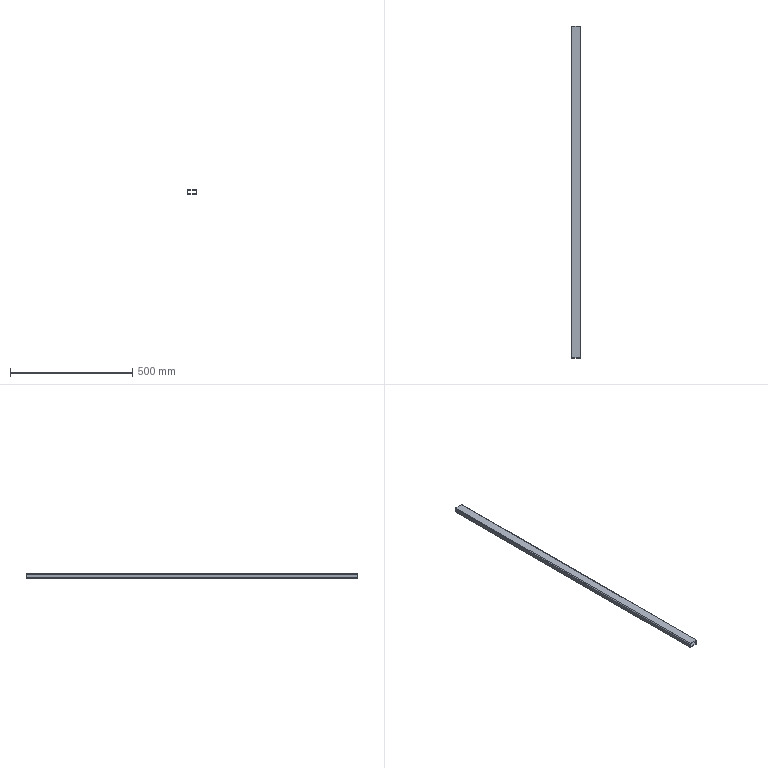Part | SolidWorks | features Extrusion 1 | 1 solid | 18 faces | box 40 x 1360 x 20 mm | volume 334231 mm3 | plane 10 | cylinder 8 | commonest cylinder face diameters 2.3 x4 6.9 x4
STEP:
#1=CARTESIAN_POINT('',(20.,1360.,-6.55));
#2=VERTEX_POINT('',#1);
#3=CARTESIAN_POINT('',(16.55,1360.,-10.));
#4=VERTEX_POINT('',#3);
#5=CARTESIAN_POINT('',(16.55,1360.,-6.55));
#6=DIRECTION('',(0.,1.,0.));
#7=DIRECTION('',(0.,0.,-1.));
#8=AXIS2_PLACEMENT_3D('',#5,#6,#7);
#9=CIRCLE('',#8,3.45);
#10=EDGE_CURVE('',#2,#4,#9,.T.);
#11=ORIENTED_EDGE('',*,*,#10,.T.);
#12=CARTESIAN_POINT('',(-16.55,1360.,-10.));
#13=VERTEX_POINT('',#12);
#14=CARTESIAN_POINT('',(-16.55,1360.,-10.));
#15=DIRECTION('',(-1.,0.,0.));
#16=VECTOR('',#15,1000.);
#17=LINE('',#14,#16);
#18=EDGE_CURVE('',#4,#13,#17,.T.);
#19=ORIENTED_EDGE('',*,*,#18,.T.);
#20=CARTESIAN_POINT('',(-20.,1360.,-6.55));
#21=VERTEX_POINT('',#20);
#22=CARTESIAN_POINT('',(-16.55,1360.,-6.55));
#23=DIRECTION('',(0.,1.,0.));
#24=DIRECTION('',(0.,0.,-1.));
#25=AXIS2_PLACEMENT_3D('',#22,#23,#24);
#26=CIRCLE('',#25,3.45);
#27=EDGE_CURVE('',#13,#21,#26,.T.);
#28=ORIENTED_EDGE('',*,*,#27,.T.);
#29=CARTESIAN_POINT('',(-20.,1360.,6.55));
#30=VERTEX_POINT('',#29);
#31=CARTESIAN_POINT('',(-20.,1360.,6.55));
#32=DIRECTION('',(0.,0.,1.));
#33=VECTOR('',#32,1000.);
#34=LINE('',#31,#33);
#35=EDGE_CURVE('',#21,#30,#34,.T.);
#36=ORIENTED_EDGE('',*,*,#35,.T.);
#37=CARTESIAN_POINT('',(-16.55,1360.,10.));
#38=VERTEX_POINT('',#37);
#39=CARTESIAN_POINT('',(-16.55,1360.,6.55));
#40=DIRECTION('',(0.,1.,0.));
#41=DIRECTION('',(0.,0.,-1.));
#42=AXIS2_PLACEMENT_3D('',#39,#40,#41);
#43=CIRCLE('',#42,3.45);
#44=EDGE_CURVE('',#30,#38,#43,.T.);
#45=ORIENTED_EDGE('',*,*,#44,.T.);
#46=CARTESIAN_POINT('',(16.55,1360.,10.));
#47=VERTEX_POINT('',#46);
#48=CARTESIAN_POINT('',(-16.55,1360.,10.));
#49=DIRECTION('',(1.,0.,0.));
#50=VECTOR('',#49,1000.);
#51=LINE('',#48,#50);
#52=EDGE_CURVE('',#38,#47,#51,.T.);
#53=ORIENTED_EDGE('',*,*,#52,.T.);
#54=CARTESIAN_POINT('',(20.,1360.,6.55));
#55=VERTEX_POINT('',#54);
#56=CARTESIAN_POINT('',(16.55,1360.,6.55));
#57=DIRECTION('',(0.,1.,0.));
#58=DIRECTION('',(0.,0.,1.));
#59=AXIS2_PLACEMENT_3D('',#56,#57,#58);
#60=CIRCLE('',#59,3.45);
#61=EDGE_CURVE('',#47,#55,#60,.T.);
#62=ORIENTED_EDGE('',*,*,#61,.T.);
#63=CARTESIAN_POINT('',(20.,1360.,6.55));
#64=DIRECTION('',(0.,0.,-1.));
#65=VECTOR('',#64,1000.);
#66=LINE('',#63,#65);
#67=EDGE_CURVE('',#55,#2,#66,.T.);
#68=ORIENTED_EDGE('',*,*,#67,.T.);
#69=EDGE_LOOP('',(#11,#19,#28,#36,#45,#53,#62,#68));
#70=FACE_OUTER_BOUND('',#69,.T.);
#71=CARTESIAN_POINT('',(-17.7,1360.,6.55));
#72=VERTEX_POINT('',#71);
#73=CARTESIAN_POINT('',(-16.55,1360.,7.7));
#74=VERTEX_POINT('',#73);
#75=CARTESIAN_POINT('',(-16.55,1360.,6.55));
#76=DIRECTION('',(0.,1.,0.));
#77=DIRECTION('',(0.,0.,-1.));
#78=AXIS2_PLACEMENT_3D('',#75,#76,#77);
#79=CIRCLE('',#78,1.15);
#80=EDGE_CURVE('',#72,#74,#79,.T.);
#81=ORIENTED_EDGE('',*,*,#80,.F.);
#82=CARTESIAN_POINT('',(-17.7,1360.,-6.55));
#83=VERTEX_POINT('',#82);
#84=CARTESIAN_POINT('',(-17.7,1360.,6.55));
#85=DIRECTION('',(0.,0.,1.));
#86=VECTOR('',#85,1000.);
#87=LINE('',#84,#86);
#88=EDGE_CURVE('',#83,#72,#87,.T.);
#89=ORIENTED_EDGE('',*,*,#88,.F.);
#90=CARTESIAN_POINT('',(-16.55,1360.,-7.7));
#91=VERTEX_POINT('',#90);
#92=CARTESIAN_POINT('',(-16.55,1360.,-6.55));
#93=DIRECTION('',(0.,1.,0.));
#94=DIRECTION('',(0.,0.,-1.));
#95=AXIS2_PLACEMENT_3D('',#92,#93,#94);
#96=CIRCLE('',#95,1.15);
#97=EDGE_CURVE('',#91,#83,#96,.T.);
#98=ORIENTED_EDGE('',*,*,#97,.F.);
#99=CARTESIAN_POINT('',(16.55,1360.,-7.7));
#100=VERTEX_POINT('',#99);
#101=CARTESIAN_POINT('',(-16.55,1360.,-7.7));
#102=DIRECTION('',(-1.,0.,0.));
#103=VECTOR('',#102,1000.);
#104=LINE('',#101,#103);
#105=EDGE_CURVE('',#100,#91,#104,.T.);
#106=ORIENTED_EDGE('',*,*,#105,.F.);
#107=CARTESIAN_POINT('',(17.7,1360.,-6.55));
#108=VERTEX_POINT('',#107);
#109=CARTESIAN_POINT('',(16.55,1360.,-6.55));
#110=DIRECTION('',(0.,1.,0.));
#111=DIRECTION('',(0.,0.,-1.));
#112=AXIS2_PLACEMENT_3D('',#109,#110,#111);
#113=CIRCLE('',#112,1.15);
#114=EDGE_CURVE('',#108,#100,#113,.T.);
#115=ORIENTED_EDGE('',*,*,#114,.F.);
#116=CARTESIAN_POINT('',(17.7,1360.,6.55));
#117=VERTEX_POINT('',#116);
#118=CARTESIAN_POINT('',(17.7,1360.,6.55));
#119=DIRECTION('',(0.,0.,-1.));
#120=VECTOR('',#119,1000.);
#121=LINE('',#118,#120);
#122=EDGE_CURVE('',#117,#108,#121,.T.);
#123=ORIENTED_EDGE('',*,*,#122,.F.);
#124=CARTESIAN_POINT('',(16.55,1360.,7.7));
#125=VERTEX_POINT('',#124);
#126=CARTESIAN_POINT('',(16.55,1360.,6.55));
#127=DIRECTION('',(0.,1.,0.));
#128=DIRECTION('',(0.,0.,1.));
#129=AXIS2_PLACEMENT_3D('',#126,#127,#128);
#130=CIRCLE('',#129,1.15);
#131=EDGE_CURVE('',#125,#117,#130,.T.);
#132=ORIENTED_EDGE('',*,*,#131,.F.);
#133=CARTESIAN_POINT('',(-16.55,1360.,7.7));
#134=DIRECTION('',(1.,0.,0.));
#135=VECTOR('',#134,1000.);
#136=LINE('',#133,#135);
#137=EDGE_CURVE('',#74,#125,#136,.T.);
#138=ORIENTED_EDGE('',*,*,#137,.F.);
#139=EDGE_LOOP('',(#81,#89,#98,#106,#115,#123,#132,#138));
#140=FACE_BOUND('',#139,.T.);
#141=CARTESIAN_POINT('',(16.55,1360.,-6.55));
#142=DIRECTION('',(0.,-1.,0.));
#143=DIRECTION('',(0.,0.,-1.));
#144=AXIS2_PLACEMENT_3D('',#141,#142,#143);
#145=PLANE('',#144);
#146=ADVANCED_FACE('',(#70,#140),#145,.F.);
#147=CARTESIAN_POINT('',(20.,0.,-6.55));
#148=VERTEX_POINT('',#147);
#149=CARTESIAN_POINT('',(16.55,0.,-10.));
#150=VERTEX_POINT('',#149);
#151=CARTESIAN_POINT('',(16.55,0.,-6.55));
#152=DIRECTION('',(0.,1.,0.));
#153=DIRECTION('',(0.,0.,-1.));
#154=AXIS2_PLACEMENT_3D('',#151,#152,#153);
#155=CIRCLE('',#154,3.45);
#156=EDGE_CURVE('',#148,#150,#155,.T.);
#157=ORIENTED_EDGE('',*,*,#156,.F.);
#158=CARTESIAN_POINT('',(20.,0.,6.55));
#159=VERTEX_POINT('',#158);
#160=CARTESIAN_POINT('',(20.,0.,6.55));
#161=DIRECTION('',(0.,0.,-1.));
#162=VECTOR('',#161,1000.);
#163=LINE('',#160,#162);
#164=EDGE_CURVE('',#159,#148,#163,.T.);
#165=ORIENTED_EDGE('',*,*,#164,.F.);
#166=CARTESIAN_POINT('',(16.55,0.,10.));
#167=VERTEX_POINT('',#166);
#168=CARTESIAN_POINT('',(16.55,0.,6.55));
#169=DIRECTION('',(0.,1.,0.));
#170=DIRECTION('',(0.,0.,1.));
#171=AXIS2_PLACEMENT_3D('',#168,#169,#170);
#172=CIRCLE('',#171,3.45);
#173=EDGE_CURVE('',#167,#159,#172,.T.);
#174=ORIENTED_EDGE('',*,*,#173,.F.);
#175=CARTESIAN_POINT('',(-16.55,0.,10.));
#176=VERTEX_POINT('',#175);
#177=CARTESIAN_POINT('',(-16.55,0.,10.));
#178=DIRECTION('',(1.,0.,0.));
#179=VECTOR('',#178,1000.);
#180=LINE('',#177,#179);
#181=EDGE_CURVE('',#176,#167,#180,.T.);
#182=ORIENTED_EDGE('',*,*,#181,.F.);
#183=CARTESIAN_POINT('',(-20.,0.,6.55));
#184=VERTEX_POINT('',#183);
#185=CARTESIAN_POINT('',(-16.55,0.,6.55));
#186=DIRECTION('',(0.,1.,0.));
#187=DIRECTION('',(0.,0.,-1.));
#188=AXIS2_PLACEMENT_3D('',#185,#186,#187);
#189=CIRCLE('',#188,3.45);
#190=EDGE_CURVE('',#184,#176,#189,.T.);
#191=ORIENTED_EDGE('',*,*,#190,.F.);
#192=CARTESIAN_POINT('',(-20.,0.,-6.55));
#193=VERTEX_POINT('',#192);
#194=CARTESIAN_POINT('',(-20.,0.,6.55));
#195=DIRECTION('',(0.,0.,1.));
#196=VECTOR('',#195,1000.);
#197=LINE('',#194,#196);
#198=EDGE_CURVE('',#193,#184,#197,.T.);
#199=ORIENTED_EDGE('',*,*,#198,.F.);
#200=CARTESIAN_POINT('',(-16.55,0.,-10.));
#201=VERTEX_POINT('',#200);
#202=CARTESIAN_POINT('',(-16.55,0.,-6.55));
#203=DIRECTION('',(0.,1.,0.));
#204=DIRECTION('',(0.,0.,-1.));
#205=AXIS2_PLACEMENT_3D('',#202,#203,#204);
#206=CIRCLE('',#205,3.45);
#207=EDGE_CURVE('',#201,#193,#206,.T.);
#208=ORIENTED_EDGE('',*,*,#207,.F.);
#209=CARTESIAN_POINT('',(-16.55,0.,-10.));
#210=DIRECTION('',(-1.,0.,0.));
#211=VECTOR('',#210,1000.);
#212=LINE('',#209,#211);
#213=EDGE_CURVE('',#150,#201,#212,.T.);
#214=ORIENTED_EDGE('',*,*,#213,.F.);
#215=EDGE_LOOP('',(#157,#165,#174,#182,#191,#199,#208,#214));
#216=FACE_OUTER_BOUND('',#215,.T.);
#217=CARTESIAN_POINT('',(-17.7,0.,-6.55));
#218=VERTEX_POINT('',#217);
#219=CARTESIAN_POINT('',(-17.7,0.,6.55));
#220=VERTEX_POINT('',#219);
#221=CARTESIAN_POINT('',(-17.7,0.,6.55));
#222=DIRECTION('',(0.,0.,1.));
#223=VECTOR('',#222,1000.);
#224=LINE('',#221,#223);
#225=EDGE_CURVE('',#218,#220,#224,.T.);
#226=ORIENTED_EDGE('',*,*,#225,.T.);
#227=CARTESIAN_POINT('',(-16.55,0.,7.7));
#228=VERTEX_POINT('',#227);
#229=CARTESIAN_POINT('',(-16.55,0.,6.55));
#230=DIRECTION('',(0.,1.,0.));
#231=DIRECTION('',(0.,0.,-1.));
#232=AXIS2_PLACEMENT_3D('',#229,#230,#231);
#233=CIRCLE('',#232,1.15);
#234=EDGE_CURVE('',#220,#228,#233,.T.);
#235=ORIENTED_EDGE('',*,*,#234,.T.);
#236=CARTESIAN_POINT('',(16.55,0.,7.7));
#237=VERTEX_POINT('',#236);
#238=CARTESIAN_POINT('',(-16.55,0.,7.7));
#239=DIRECTION('',(1.,0.,0.));
#240=VECTOR('',#239,1000.);
#241=LINE('',#238,#240);
#242=EDGE_CURVE('',#228,#237,#241,.T.);
#243=ORIENTED_EDGE('',*,*,#242,.T.);
#244=CARTESIAN_POINT('',(17.7,0.,6.55));
#245=VERTEX_POINT('',#244);
#246=CARTESIAN_POINT('',(16.55,0.,6.55));
#247=DIRECTION('',(0.,1.,0.));
#248=DIRECTION('',(0.,0.,1.));
#249=AXIS2_PLACEMENT_3D('',#246,#247,#248);
#250=CIRCLE('',#249,1.15);
#251=EDGE_CURVE('',#237,#245,#250,.T.);
#252=ORIENTED_EDGE('',*,*,#251,.T.);
#253=CARTESIAN_POINT('',(17.7,0.,-6.55));
#254=VERTEX_POINT('',#253);
#255=CARTESIAN_POINT('',(17.7,0.,6.55));
#256=DIRECTION('',(0.,0.,-1.));
#257=VECTOR('',#256,1000.);
#258=LINE('',#255,#257);
#259=EDGE_CURVE('',#245,#254,#258,.T.);
#260=ORIENTED_EDGE('',*,*,#259,.T.);
#261=CARTESIAN_POINT('',(16.55,0.,-7.7));
#262=VERTEX_POINT('',#261);
#263=CARTESIAN_POINT('',(16.55,0.,-6.55));
#264=DIRECTION('',(0.,1.,0.));
#265=DIRECTION('',(0.,0.,-1.));
#266=AXIS2_PLACEMENT_3D('',#263,#264,#265);
#267=CIRCLE('',#266,1.15);
#268=EDGE_CURVE('',#254,#262,#267,.T.);
#269=ORIENTED_EDGE('',*,*,#268,.T.);
#270=CARTESIAN_POINT('',(-16.55,0.,-7.7));
#271=VERTEX_POINT('',#270);
#272=CARTESIAN_POINT('',(-16.55,0.,-7.7));
#273=DIRECTION('',(-1.,0.,0.));
#274=VECTOR('',#273,1000.);
#275=LINE('',#272,#274);
#276=EDGE_CURVE('',#262,#271,#275,.T.);
#277=ORIENTED_EDGE('',*,*,#276,.T.);
#278=CARTESIAN_POINT('',(-16.55,0.,-6.55));
#279=DIRECTION('',(0.,1.,0.));
#280=DIRECTION('',(0.,0.,-1.));
#281=AXIS2_PLACEMENT_3D('',#278,#279,#280);
#282=CIRCLE('',#281,1.15);
#283=EDGE_CURVE('',#271,#218,#282,.T.);
#284=ORIENTED_EDGE('',*,*,#283,.T.);
#285=EDGE_LOOP('',(#226,#235,#243,#252,#260,#269,#277,#284));
#286=FACE_BOUND('',#285,.T.);
#287=CARTESIAN_POINT('',(16.55,0.,-6.55));
#288=DIRECTION('',(0.,-1.,0.));
#289=DIRECTION('',(0.,0.,-1.));
#290=AXIS2_PLACEMENT_3D('',#287,#288,#289);
#291=PLANE('',#290);
#292=ADVANCED_FACE('',(#216,#286),#291,.T.);
#293=ORIENTED_EDGE('',*,*,#156,.T.);
#294=CARTESIAN_POINT('',(16.55,1360.,-10.));
#295=DIRECTION('',(0.,-1.,0.));
#296=VECTOR('',#295,1000.);
#297=LINE('',#294,#296);
#298=EDGE_CURVE('',#4,#150,#297,.T.);
#299=ORIENTED_EDGE('',*,*,#298,.F.);
#300=ORIENTED_EDGE('',*,*,#10,.F.);
#301=CARTESIAN_POINT('',(20.,1360.,-6.55));
#302=DIRECTION('',(0.,-1.,0.));
#303=VECTOR('',#302,1000.);
#304=LINE('',#301,#303);
#305=EDGE_CURVE('',#2,#148,#304,.T.);
#306=ORIENTED_EDGE('',*,*,#305,.T.);
#307=EDGE_LOOP('',(#293,#299,#300,#306));
#308=FACE_OUTER_BOUND('',#307,.T.);
#309=CARTESIAN_POINT('',(16.55,1360.,-6.55));
#310=DIRECTION('',(0.,-1.,0.));
#311=DIRECTION('',(0.,0.,-1.));
#312=AXIS2_PLACEMENT_3D('',#309,#310,#311);
#313=CYLINDRICAL_SURFACE('',#312,3.45);
#314=ADVANCED_FACE('',(#308),#313,.T.);
#315=ORIENTED_EDGE('',*,*,#213,.T.);
#316=CARTESIAN_POINT('',(-16.55,1360.,-10.));
#317=DIRECTION('',(0.,-1.,0.));
#318=VECTOR('',#317,1000.);
#319=LINE('',#316,#318);
#320=EDGE_CURVE('',#13,#201,#319,.T.);
#321=ORIENTED_EDGE('',*,*,#320,.F.);
#322=ORIENTED_EDGE('',*,*,#18,.F.);
#323=ORIENTED_EDGE('',*,*,#298,.T.);
#324=EDGE_LOOP('',(#315,#321,#322,#323));
#325=FACE_OUTER_BOUND('',#324,.T.);
#326=CARTESIAN_POINT('',(-16.55,1360.,-10.));
#327=DIRECTION('',(0.,0.,1.));
#328=DIRECTION('',(1.,0.,0.));
#329=AXIS2_PLACEMENT_3D('',#326,#327,#328);
#330=PLANE('',#329);
#331=ADVANCED_FACE('',(#325),#330,.F.);
#332=ORIENTED_EDGE('',*,*,#207,.T.);
#333=CARTESIAN_POINT('',(-20.,1360.,-6.55));
#334=DIRECTION('',(0.,-1.,0.));
#335=VECTOR('',#334,1000.);
#336=LINE('',#333,#335);
#337=EDGE_CURVE('',#21,#193,#336,.T.);
#338=ORIENTED_EDGE('',*,*,#337,.F.);
#339=ORIENTED_EDGE('',*,*,#27,.F.);
#340=ORIENTED_EDGE('',*,*,#320,.T.);
#341=EDGE_LOOP('',(#332,#338,#339,#340));
#342=FACE_OUTER_BOUND('',#341,.T.);
#343=CARTESIAN_POINT('',(-16.55,1360.,-6.55));
#344=DIRECTION('',(0.,-1.,0.));
#345=DIRECTION('',(0.,0.,-1.));
#346=AXIS2_PLACEMENT_3D('',#343,#344,#345);
#347=CYLINDRICAL_SURFACE('',#346,3.45);
#348=ADVANCED_FACE('',(#342),#347,.T.);
#349=ORIENTED_EDGE('',*,*,#198,.T.);
#350=CARTESIAN_POINT('',(-20.,1360.,6.55));
#351=DIRECTION('',(0.,-1.,0.));
#352=VECTOR('',#351,1000.);
#353=LINE('',#350,#352);
#354=EDGE_CURVE('',#30,#184,#353,.T.);
#355=ORIENTED_EDGE('',*,*,#354,.F.);
#356=ORIENTED_EDGE('',*,*,#35,.F.);
#357=ORIENTED_EDGE('',*,*,#337,.T.);
#358=EDGE_LOOP('',(#349,#355,#356,#357));
#359=FACE_OUTER_BOUND('',#358,.T.);
#360=CARTESIAN_POINT('',(-20.,1360.,6.55));
#361=DIRECTION('',(1.,0.,0.));
#362=DIRECTION('',(0.,0.,-1.));
#363=AXIS2_PLACEMENT_3D('',#360,#361,#362);
#364=PLANE('',#363);
#365=ADVANCED_FACE('',(#359),#364,.F.);
#366=ORIENTED_EDGE('',*,*,#190,.T.);
#367=CARTESIAN_POINT('',(-16.55,1360.,10.));
#368=DIRECTION('',(0.,-1.,0.));
#369=VECTOR('',#368,1000.);
#370=LINE('',#367,#369);
#371=EDGE_CURVE('',#38,#176,#370,.T.);
#372=ORIENTED_EDGE('',*,*,#371,.F.);
#373=ORIENTED_EDGE('',*,*,#44,.F.);
#374=ORIENTED_EDGE('',*,*,#354,.T.);
#375=EDGE_LOOP('',(#366,#372,#373,#374));
#376=FACE_OUTER_BOUND('',#375,.T.);
#377=CARTESIAN_POINT('',(-16.55,1360.,6.55));
#378=DIRECTION('',(0.,-1.,0.));
#379=DIRECTION('',(0.,0.,-1.));
#380=AXIS2_PLACEMENT_3D('',#377,#378,#379);
#381=CYLINDRICAL_SURFACE('',#380,3.45);
#382=ADVANCED_FACE('',(#376),#381,.T.);
#383=ORIENTED_EDGE('',*,*,#181,.T.);
#384=CARTESIAN_POINT('',(16.55,1360.,10.));
#385=DIRECTION('',(0.,-1.,0.));
#386=VECTOR('',#385,1000.);
#387=LINE('',#384,#386);
#388=EDGE_CURVE('',#47,#167,#387,.T.);
#389=ORIENTED_EDGE('',*,*,#388,.F.);
#390=ORIENTED_EDGE('',*,*,#52,.F.);
#391=ORIENTED_EDGE('',*,*,#371,.T.);
#392=EDGE_LOOP('',(#383,#389,#390,#391));
#393=FACE_OUTER_BOUND('',#392,.T.);
#394=CARTESIAN_POINT('',(-16.55,1360.,10.));
#395=DIRECTION('',(0.,0.,-1.));
#396=DIRECTION('',(-1.,0.,0.));
#397=AXIS2_PLACEMENT_3D('',#394,#395,#396);
#398=PLANE('',#397);
#399=ADVANCED_FACE('',(#393),#398,.F.);
#400=ORIENTED_EDGE('',*,*,#173,.T.);
#401=CARTESIAN_POINT('',(20.,1360.,6.55));
#402=DIRECTION('',(0.,-1.,0.));
#403=VECTOR('',#402,1000.);
#404=LINE('',#401,#403);
#405=EDGE_CURVE('',#55,#159,#404,.T.);
#406=ORIENTED_EDGE('',*,*,#405,.F.);
#407=ORIENTED_EDGE('',*,*,#61,.F.);
#408=ORIENTED_EDGE('',*,*,#388,.T.);
#409=EDGE_LOOP('',(#400,#406,#407,#408));
#410=FACE_OUTER_BOUND('',#409,.T.);
#411=CARTESIAN_POINT('',(16.55,1360.,6.55));
#412=DIRECTION('',(0.,-1.,0.));
#413=DIRECTION('',(0.,0.,-1.));
#414=AXIS2_PLACEMENT_3D('',#411,#412,#413);
#415=CYLINDRICAL_SURFACE('',#414,3.45);
#416=ADVANCED_FACE('',(#410),#415,.T.);
#417=ORIENTED_EDGE('',*,*,#164,.T.);
#418=ORIENTED_EDGE('',*,*,#305,.F.);
#419=ORIENTED_EDGE('',*,*,#67,.F.);
#420=ORIENTED_EDGE('',*,*,#405,.T.);
#421=EDGE_LOOP('',(#417,#418,#419,#420));
#422=FACE_OUTER_BOUND('',#421,.T.);
#423=CARTESIAN_POINT('',(20.,1360.,6.55));
#424=DIRECTION('',(-1.,0.,0.));
#425=DIRECTION('',(0.,0.,1.));
#426=AXIS2_PLACEMENT_3D('',#423,#424,#425);
#427=PLANE('',#426);
#428=ADVANCED_FACE('',(#422),#427,.F.);
#429=ORIENTED_EDGE('',*,*,#234,.F.);
#430=CARTESIAN_POINT('',(-17.7,1360.,6.55));
#431=DIRECTION('',(0.,-1.,0.));
#432=VECTOR('',#431,1000.);
#433=LINE('',#430,#432);
#434=EDGE_CURVE('',#72,#220,#433,.T.);
#435=ORIENTED_EDGE('',*,*,#434,.F.);
#436=ORIENTED_EDGE('',*,*,#80,.T.);
#437=CARTESIAN_POINT('',(-16.55,1360.,7.7));
#438=DIRECTION('',(0.,-1.,0.));
#439=VECTOR('',#438,1000.);
#440=LINE('',#437,#439);
#441=EDGE_CURVE('',#74,#228,#440,.T.);
#442=ORIENTED_EDGE('',*,*,#441,.T.);
#443=EDGE_LOOP('',(#429,#435,#436,#442));
#444=FACE_OUTER_BOUND('',#443,.T.);
#445=CARTESIAN_POINT('',(-16.55,1360.,6.55));
#446=DIRECTION('',(0.,-1.,0.));
#447=DIRECTION('',(0.,0.,-1.));
#448=AXIS2_PLACEMENT_3D('',#445,#446,#447);
#449=CYLINDRICAL_SURFACE('',#448,1.15);
#450=ADVANCED_FACE('',(#444),#449,.F.);
#451=ORIENTED_EDGE('',*,*,#242,.F.);
#452=ORIENTED_EDGE('',*,*,#441,.F.);
#453=ORIENTED_EDGE('',*,*,#137,.T.);
#454=CARTESIAN_POINT('',(16.55,1360.,7.7));
#455=DIRECTION('',(0.,-1.,0.));
#456=VECTOR('',#455,1000.);
#457=LINE('',#454,#456);
#458=EDGE_CURVE('',#125,#237,#457,.T.);
#459=ORIENTED_EDGE('',*,*,#458,.T.);
#460=EDGE_LOOP('',(#451,#452,#453,#459));
#461=FACE_OUTER_BOUND('',#460,.T.);
#462=CARTESIAN_POINT('',(-16.55,1360.,7.7));
#463=DIRECTION('',(0.,0.,-1.));
#464=DIRECTION('',(-1.,0.,0.));
#465=AXIS2_PLACEMENT_3D('',#462,#463,#464);
#466=PLANE('',#465);
#467=ADVANCED_FACE('',(#461),#466,.T.);
#468=ORIENTED_EDGE('',*,*,#251,.F.);
#469=ORIENTED_EDGE('',*,*,#458,.F.);
#470=ORIENTED_EDGE('',*,*,#131,.T.);
#471=CARTESIAN_POINT('',(17.7,1360.,6.55));
#472=DIRECTION('',(0.,-1.,0.));
#473=VECTOR('',#472,1000.);
#474=LINE('',#471,#473);
#475=EDGE_CURVE('',#117,#245,#474,.T.);
#476=ORIENTED_EDGE('',*,*,#475,.T.);
#477=EDGE_LOOP('',(#468,#469,#470,#476));
#478=FACE_OUTER_BOUND('',#477,.T.);
#479=CARTESIAN_POINT('',(16.55,1360.,6.55));
#480=DIRECTION('',(0.,-1.,0.));
#481=DIRECTION('',(0.,0.,-1.));
#482=AXIS2_PLACEMENT_3D('',#479,#480,#481);
#483=CYLINDRICAL_SURFACE('',#482,1.15);
#484=ADVANCED_FACE('',(#478),#483,.F.);
#485=ORIENTED_EDGE('',*,*,#259,.F.);
#486=ORIENTED_EDGE('',*,*,#475,.F.);
#487=ORIENTED_EDGE('',*,*,#122,.T.);
#488=CARTESIAN_POINT('',(17.7,1360.,-6.55));
#489=DIRECTION('',(0.,-1.,0.));
#490=VECTOR('',#489,1000.);
#491=LINE('',#488,#490);
#492=EDGE_CURVE('',#108,#254,#491,.T.);
#493=ORIENTED_EDGE('',*,*,#492,.T.);
#494=EDGE_LOOP('',(#485,#486,#487,#493));
#495=FACE_OUTER_BOUND('',#494,.T.);
#496=CARTESIAN_POINT('',(17.7,1360.,6.55));
#497=DIRECTION('',(-1.,0.,0.));
#498=DIRECTION('',(0.,0.,1.));
#499=AXIS2_PLACEMENT_3D('',#496,#497,#498);
#500=PLANE('',#499);
#501=ADVANCED_FACE('',(#495),#500,.T.);
#502=ORIENTED_EDGE('',*,*,#268,.F.);
#503=ORIENTED_EDGE('',*,*,#492,.F.);
#504=ORIENTED_EDGE('',*,*,#114,.T.);
#505=CARTESIAN_POINT('',(16.55,1360.,-7.7));
#506=DIRECTION('',(0.,-1.,0.));
#507=VECTOR('',#506,1000.);
#508=LINE('',#505,#507);
#509=EDGE_CURVE('',#100,#262,#508,.T.);
#510=ORIENTED_EDGE('',*,*,#509,.T.);
#511=EDGE_LOOP('',(#502,#503,#504,#510));
#512=FACE_OUTER_BOUND('',#511,.T.);
#513=CARTESIAN_POINT('',(16.55,1360.,-6.55));
#514=DIRECTION('',(0.,-1.,0.));
#515=DIRECTION('',(0.,0.,-1.));
#516=AXIS2_PLACEMENT_3D('',#513,#514,#515);
#517=CYLINDRICAL_SURFACE('',#516,1.15);
#518=ADVANCED_FACE('',(#512),#517,.F.);
#519=ORIENTED_EDGE('',*,*,#276,.F.);
#520=ORIENTED_EDGE('',*,*,#509,.F.);
#521=ORIENTED_EDGE('',*,*,#105,.T.);
#522=CARTESIAN_POINT('',(-16.55,1360.,-7.7));
#523=DIRECTION('',(0.,-1.,0.));
#524=VECTOR('',#523,1000.);
#525=LINE('',#522,#524);
#526=EDGE_CURVE('',#91,#271,#525,.T.);
#527=ORIENTED_EDGE('',*,*,#526,.T.);
#528=EDGE_LOOP('',(#519,#520,#521,#527));
#529=FACE_OUTER_BOUND('',#528,.T.);
#530=CARTESIAN_POINT('',(-16.55,1360.,-7.7));
#531=DIRECTION('',(0.,0.,1.));
#532=DIRECTION('',(1.,0.,0.));
#533=AXIS2_PLACEMENT_3D('',#530,#531,#532);
#534=PLANE('',#533);
#535=ADVANCED_FACE('',(#529),#534,.T.);
#536=ORIENTED_EDGE('',*,*,#283,.F.);
#537=ORIENTED_EDGE('',*,*,#526,.F.);
#538=ORIENTED_EDGE('',*,*,#97,.T.);
#539=CARTESIAN_POINT('',(-17.7,1360.,-6.55));
#540=DIRECTION('',(0.,-1.,0.));
#541=VECTOR('',#540,1000.);
#542=LINE('',#539,#541);
#543=EDGE_CURVE('',#83,#218,#542,.T.);
#544=ORIENTED_EDGE('',*,*,#543,.T.);
#545=EDGE_LOOP('',(#536,#537,#538,#544));
#546=FACE_OUTER_BOUND('',#545,.T.);
#547=CARTESIAN_POINT('',(-16.55,1360.,-6.55));
#548=DIRECTION('',(0.,-1.,0.));
#549=DIRECTION('',(0.,0.,-1.));
#550=AXIS2_PLACEMENT_3D('',#547,#548,#549);
#551=CYLINDRICAL_SURFACE('',#550,1.15);
#552=ADVANCED_FACE('',(#546),#551,.F.);
#553=ORIENTED_EDGE('',*,*,#225,.F.);
#554=ORIENTED_EDGE('',*,*,#543,.F.);
#555=ORIENTED_EDGE('',*,*,#88,.T.);
#556=ORIENTED_EDGE('',*,*,#434,.T.);
#557=EDGE_LOOP('',(#553,#554,#555,#556));
#558=FACE_OUTER_BOUND('',#557,.T.);
#559=CARTESIAN_POINT('',(-17.7,1360.,6.55));
#560=DIRECTION('',(1.,0.,0.));
#561=DIRECTION('',(0.,0.,-1.));
#562=AXIS2_PLACEMENT_3D('',#559,#560,#561);
#563=PLANE('',#562);
#564=ADVANCED_FACE('',(#558),#563,.T.);
#565=CLOSED_SHELL('',(#146,#292,#314,#331,#348,#365,#382,#399,#416,#428,#450,#467,#484,#501,#518,#535,#552,#564));
#566=MANIFOLD_SOLID_BREP('',#565);
#567=CARTESIAN_POINT('',(0.,0.,0.));
#568=DIRECTION('',(0.,0.,1.));
#569=DIRECTION('',(1.,0.,0.));
#570=AXIS2_PLACEMENT_3D('',#567,#568,#569);
#571=(LENGTH_UNIT()NAMED_UNIT(*)SI_UNIT(.MILLI.,.METRE.));
#572=UNCERTAINTY_MEASURE_WITH_UNIT(LENGTH_MEASURE(0.00001),#571,'','');
#573=(NAMED_UNIT(*)PLANE_ANGLE_UNIT()SI_UNIT($,.RADIAN.));
#574=(NAMED_UNIT(*)SI_UNIT($,.STERADIAN.)SOLID_ANGLE_UNIT());
#575=(GEOMETRIC_REPRESENTATION_CONTEXT(3)GLOBAL_UNCERTAINTY_ASSIGNED_CONTEXT((#572))GLOBAL_UNIT_ASSIGNED_CONTEXT((#571,#573,#574))REPRESENTATION_CONTEXT('',''));
#576=ADVANCED_BREP_SHAPE_REPRESENTATION('',(#566,#570),#575);